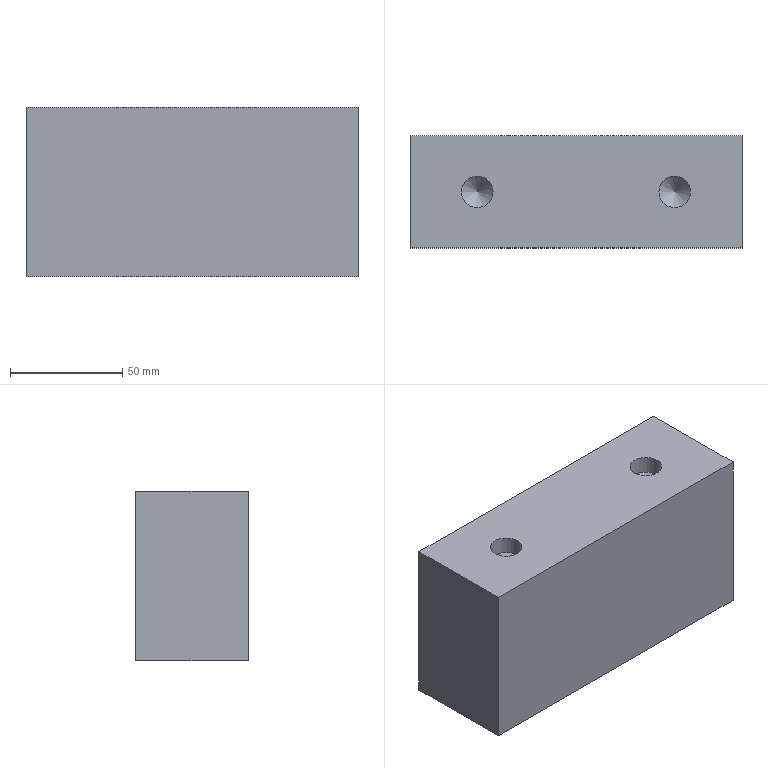Part | NX | features 3 2 | 1 solid | 10 faces | box 148 x 50 x 75.5 mm | volume 555483 mm3 | plane 6 | cylinder 2 | cone 2 | commonest cylinder face diameters 14.1 x2
STEP:
#1=CARTESIAN_POINT('',(1481.05,-647.5,256.5));
#2=VERTEX_POINT('',#1);
#3=CARTESIAN_POINT('',(1474.,-647.5,256.5));
#4=DIRECTION('',(0.,0.,-1.));
#5=DIRECTION('',(1.,0.,0.));
#6=AXIS2_PLACEMENT_3D('',#3,#4,#5);
#7=CIRCLE('',#6,7.05);
#8=EDGE_CURVE('',#2,#2,#7,.T.);
#9=ORIENTED_EDGE('',*,*,#8,.T.);
#10=EDGE_LOOP('',(#9));
#11=FACE_BOUND('',#10,.T.);
#12=CARTESIAN_POINT('',(1504.,-672.5,256.5));
#13=VERTEX_POINT('',#12);
#14=CARTESIAN_POINT('',(1356.,-672.5,256.5));
#15=VERTEX_POINT('',#14);
#16=CARTESIAN_POINT('',(927.,-672.5,256.5));
#17=DIRECTION('',(-1.,0.,0.));
#18=VECTOR('',#17,1000.);
#19=LINE('',#16,#18);
#20=EDGE_CURVE('',#13,#15,#19,.T.);
#21=ORIENTED_EDGE('',*,*,#20,.F.);
#22=CARTESIAN_POINT('',(1504.,-622.5,256.5));
#23=VERTEX_POINT('',#22);
#24=CARTESIAN_POINT('',(1504.,1367.5,256.5));
#25=DIRECTION('',(0.,1.,0.));
#26=VECTOR('',#25,1000.);
#27=LINE('',#24,#26);
#28=EDGE_CURVE('',#13,#23,#27,.T.);
#29=ORIENTED_EDGE('',*,*,#28,.T.);
#30=CARTESIAN_POINT('',(1356.,-622.5,256.5));
#31=VERTEX_POINT('',#30);
#32=CARTESIAN_POINT('',(927.,-622.5,256.5));
#33=DIRECTION('',(1.,0.,0.));
#34=VECTOR('',#33,1000.);
#35=LINE('',#32,#34);
#36=EDGE_CURVE('',#31,#23,#35,.T.);
#37=ORIENTED_EDGE('',*,*,#36,.F.);
#38=CARTESIAN_POINT('',(1356.,1367.5,256.5));
#39=DIRECTION('',(0.,-1.,0.));
#40=VECTOR('',#39,1000.);
#41=LINE('',#38,#40);
#42=EDGE_CURVE('',#31,#15,#41,.T.);
#43=ORIENTED_EDGE('',*,*,#42,.T.);
#44=EDGE_LOOP('',(#21,#29,#37,#43));
#45=FACE_BOUND('',#44,.T.);
#46=CARTESIAN_POINT('',(1393.05,-647.5,256.5));
#47=VERTEX_POINT('',#46);
#48=CARTESIAN_POINT('',(1386.,-647.5,256.5));
#49=DIRECTION('',(0.,0.,-1.));
#50=DIRECTION('',(1.,0.,0.));
#51=AXIS2_PLACEMENT_3D('',#48,#49,#50);
#52=CIRCLE('',#51,7.05);
#53=EDGE_CURVE('',#47,#47,#52,.T.);
#54=ORIENTED_EDGE('',*,*,#53,.T.);
#55=EDGE_LOOP('',(#54));
#56=FACE_BOUND('',#55,.T.);
#57=CARTESIAN_POINT('',(1120.,1367.5,256.5));
#58=DIRECTION('',(0.,0.,1.));
#59=DIRECTION('',(0.,-1.,0.));
#60=AXIS2_PLACEMENT_3D('',#57,#58,#59);
#61=PLANE('',#60);
#62=ADVANCED_FACE('',(#11,#45,#56),#61,.T.);
#63=CARTESIAN_POINT('',(1504.,-622.5,181.));
#64=VERTEX_POINT('',#63);
#65=CARTESIAN_POINT('',(1504.,-622.5,-1.5));
#66=DIRECTION('',(0.,0.,-1.));
#67=VECTOR('',#66,1000.);
#68=LINE('',#65,#67);
#69=EDGE_CURVE('',#23,#64,#68,.T.);
#70=ORIENTED_EDGE('',*,*,#69,.F.);
#71=ORIENTED_EDGE('',*,*,#28,.F.);
#72=CARTESIAN_POINT('',(1504.,-672.5,181.));
#73=VERTEX_POINT('',#72);
#74=CARTESIAN_POINT('',(1504.,-672.5,-1.5));
#75=DIRECTION('',(0.,0.,1.));
#76=VECTOR('',#75,1000.);
#77=LINE('',#74,#76);
#78=EDGE_CURVE('',#73,#13,#77,.T.);
#79=ORIENTED_EDGE('',*,*,#78,.F.);
#80=CARTESIAN_POINT('',(1504.,597.5,181.));
#81=DIRECTION('',(0.,-1.,0.));
#82=VECTOR('',#81,1000.);
#83=LINE('',#80,#82);
#84=EDGE_CURVE('',#64,#73,#83,.T.);
#85=ORIENTED_EDGE('',*,*,#84,.F.);
#86=EDGE_LOOP('',(#70,#71,#79,#85));
#87=FACE_BOUND('',#86,.T.);
#88=CARTESIAN_POINT('',(1504.,0.,218.75));
#89=DIRECTION('',(1.,0.,0.));
#90=DIRECTION('',(0.,0.,1.));
#91=AXIS2_PLACEMENT_3D('',#88,#89,#90);
#92=PLANE('',#91);
#93=ADVANCED_FACE('',(#87),#92,.T.);
#94=CARTESIAN_POINT('',(1356.,-622.5,181.));
#95=VERTEX_POINT('',#94);
#96=CARTESIAN_POINT('',(927.,-622.5,181.));
#97=DIRECTION('',(-1.,0.,0.));
#98=VECTOR('',#97,1000.);
#99=LINE('',#96,#98);
#100=EDGE_CURVE('',#64,#95,#99,.T.);
#101=ORIENTED_EDGE('',*,*,#100,.F.);
#102=ORIENTED_EDGE('',*,*,#84,.T.);
#103=CARTESIAN_POINT('',(1356.,-672.5,181.));
#104=VERTEX_POINT('',#103);
#105=CARTESIAN_POINT('',(927.,-672.5,181.));
#106=DIRECTION('',(1.,0.,0.));
#107=VECTOR('',#106,1000.);
#108=LINE('',#105,#107);
#109=EDGE_CURVE('',#104,#73,#108,.T.);
#110=ORIENTED_EDGE('',*,*,#109,.F.);
#111=CARTESIAN_POINT('',(1356.,597.5,181.));
#112=DIRECTION('',(0.,1.,0.));
#113=VECTOR('',#112,1000.);
#114=LINE('',#111,#113);
#115=EDGE_CURVE('',#104,#95,#114,.T.);
#116=ORIENTED_EDGE('',*,*,#115,.T.);
#117=EDGE_LOOP('',(#101,#102,#110,#116));
#118=FACE_BOUND('',#117,.T.);
#119=CARTESIAN_POINT('',(927.,597.5,181.));
#120=DIRECTION('',(0.,0.,-1.));
#121=DIRECTION('',(0.,-1.,0.));
#122=AXIS2_PLACEMENT_3D('',#119,#120,#121);
#123=PLANE('',#122);
#124=ADVANCED_FACE('',(#118),#123,.T.);
#125=ORIENTED_EDGE('',*,*,#36,.T.);
#126=ORIENTED_EDGE('',*,*,#69,.T.);
#127=ORIENTED_EDGE('',*,*,#100,.T.);
#128=CARTESIAN_POINT('',(1356.,-622.5,-1.5));
#129=DIRECTION('',(0.,0.,1.));
#130=VECTOR('',#129,1000.);
#131=LINE('',#128,#130);
#132=EDGE_CURVE('',#95,#31,#131,.T.);
#133=ORIENTED_EDGE('',*,*,#132,.T.);
#134=EDGE_LOOP('',(#125,#126,#127,#133));
#135=FACE_BOUND('',#134,.T.);
#136=CARTESIAN_POINT('',(927.,-622.5,-1.5));
#137=DIRECTION('',(0.,1.,0.));
#138=DIRECTION('',(0.,0.,1.));
#139=AXIS2_PLACEMENT_3D('',#136,#137,#138);
#140=PLANE('',#139);
#141=ADVANCED_FACE('',(#135),#140,.T.);
#142=ORIENTED_EDGE('',*,*,#109,.T.);
#143=ORIENTED_EDGE('',*,*,#78,.T.);
#144=ORIENTED_EDGE('',*,*,#20,.T.);
#145=CARTESIAN_POINT('',(1356.,-672.5,-1.5));
#146=DIRECTION('',(0.,0.,-1.));
#147=VECTOR('',#146,1000.);
#148=LINE('',#145,#147);
#149=EDGE_CURVE('',#15,#104,#148,.T.);
#150=ORIENTED_EDGE('',*,*,#149,.T.);
#151=EDGE_LOOP('',(#142,#143,#144,#150));
#152=FACE_BOUND('',#151,.T.);
#153=CARTESIAN_POINT('',(927.,-672.5,-1.5));
#154=DIRECTION('',(0.,-1.,0.));
#155=DIRECTION('',(0.,0.,-1.));
#156=AXIS2_PLACEMENT_3D('',#153,#154,#155);
#157=PLANE('',#156);
#158=ADVANCED_FACE('',(#152),#157,.T.);
#159=ORIENTED_EDGE('',*,*,#132,.F.);
#160=ORIENTED_EDGE('',*,*,#115,.F.);
#161=ORIENTED_EDGE('',*,*,#149,.F.);
#162=ORIENTED_EDGE('',*,*,#42,.F.);
#163=EDGE_LOOP('',(#159,#160,#161,#162));
#164=FACE_BOUND('',#163,.T.);
#165=CARTESIAN_POINT('',(1356.,-551.349,218.75));
#166=DIRECTION('',(-1.,0.,0.));
#167=DIRECTION('',(0.,0.,-1.));
#168=AXIS2_PLACEMENT_3D('',#165,#166,#167);
#169=PLANE('',#168);
#170=ADVANCED_FACE('',(#164),#169,.T.);
#171=CARTESIAN_POINT('',(1466.95,-647.5,248.55));
#172=VERTEX_POINT('',#171);
#173=CARTESIAN_POINT('',(1474.,-647.5,248.55));
#174=DIRECTION('',(0.,0.,-1.));
#175=DIRECTION('',(-1.,0.,0.));
#176=AXIS2_PLACEMENT_3D('',#173,#174,#175);
#177=CIRCLE('',#176,7.05);
#178=EDGE_CURVE('',#172,#172,#177,.T.);
#179=ORIENTED_EDGE('',*,*,#178,.T.);
#180=EDGE_LOOP('',(#179));
#181=FACE_BOUND('',#180,.T.);
#182=ORIENTED_EDGE('',*,*,#8,.F.);
#183=EDGE_LOOP('',(#182));
#184=FACE_BOUND('',#183,.T.);
#185=CARTESIAN_POINT('',(1474.,-647.5,256.5));
#186=DIRECTION('',(0.,0.,-1.));
#187=DIRECTION('',(-1.,0.,0.));
#188=AXIS2_PLACEMENT_3D('',#185,#186,#187);
#189=CYLINDRICAL_SURFACE('',#188,7.05);
#190=ADVANCED_FACE('',(#181,#184),#189,.F.);
#191=CARTESIAN_POINT('',(1474.,-647.5,241.5));
#192=VERTEX_POINT('',#191);
#193=VERTEX_LOOP('',#192);
#194=FACE_BOUND('',#193,.T.);
#195=ORIENTED_EDGE('',*,*,#178,.F.);
#196=EDGE_LOOP('',(#195));
#197=FACE_BOUND('',#196,.T.);
#198=CARTESIAN_POINT('',(1474.,-647.5,248.55));
#199=DIRECTION('',(0.,0.,1.));
#200=DIRECTION('',(-1.,0.,0.));
#201=AXIS2_PLACEMENT_3D('',#198,#199,#200);
#202=CONICAL_SURFACE('',#201,7.05,0.7854);
#203=ADVANCED_FACE('',(#194,#197),#202,.F.);
#204=CARTESIAN_POINT('',(1378.95,-647.5,248.55));
#205=VERTEX_POINT('',#204);
#206=CARTESIAN_POINT('',(1386.,-647.5,248.55));
#207=DIRECTION('',(0.,0.,-1.));
#208=DIRECTION('',(-1.,0.,0.));
#209=AXIS2_PLACEMENT_3D('',#206,#207,#208);
#210=CIRCLE('',#209,7.05);
#211=EDGE_CURVE('',#205,#205,#210,.T.);
#212=ORIENTED_EDGE('',*,*,#211,.T.);
#213=EDGE_LOOP('',(#212));
#214=FACE_BOUND('',#213,.T.);
#215=ORIENTED_EDGE('',*,*,#53,.F.);
#216=EDGE_LOOP('',(#215));
#217=FACE_BOUND('',#216,.T.);
#218=CARTESIAN_POINT('',(1386.,-647.5,256.5));
#219=DIRECTION('',(0.,0.,-1.));
#220=DIRECTION('',(-1.,0.,0.));
#221=AXIS2_PLACEMENT_3D('',#218,#219,#220);
#222=CYLINDRICAL_SURFACE('',#221,7.05);
#223=ADVANCED_FACE('',(#214,#217),#222,.F.);
#224=CARTESIAN_POINT('',(1386.,-647.5,241.5));
#225=VERTEX_POINT('',#224);
#226=VERTEX_LOOP('',#225);
#227=FACE_BOUND('',#226,.T.);
#228=ORIENTED_EDGE('',*,*,#211,.F.);
#229=EDGE_LOOP('',(#228));
#230=FACE_BOUND('',#229,.T.);
#231=CARTESIAN_POINT('',(1386.,-647.5,248.55));
#232=DIRECTION('',(0.,0.,1.));
#233=DIRECTION('',(-1.,0.,0.));
#234=AXIS2_PLACEMENT_3D('',#231,#232,#233);
#235=CONICAL_SURFACE('',#234,7.05,0.7854);
#236=ADVANCED_FACE('',(#227,#230),#235,.F.);
#237=CLOSED_SHELL('',(#62,#93,#124,#141,#158,#170,#190,#203,#223,#236));
#238=MANIFOLD_SOLID_BREP('',#237);
#239=(LENGTH_UNIT()NAMED_UNIT(*)SI_UNIT(.MILLI.,.METRE.));
#240=UNCERTAINTY_MEASURE_WITH_UNIT(LENGTH_MEASURE(0.00001),#239,'','');
#241=(NAMED_UNIT(*)PLANE_ANGLE_UNIT()SI_UNIT($,.RADIAN.));
#242=(NAMED_UNIT(*)SI_UNIT($,.STERADIAN.)SOLID_ANGLE_UNIT());
#243=(GEOMETRIC_REPRESENTATION_CONTEXT(3)GLOBAL_UNCERTAINTY_ASSIGNED_CONTEXT((#240))GLOBAL_UNIT_ASSIGNED_CONTEXT((#239,#241,#242))REPRESENTATION_CONTEXT('',''));
#244=ADVANCED_BREP_SHAPE_REPRESENTATION('',(#238),#243);